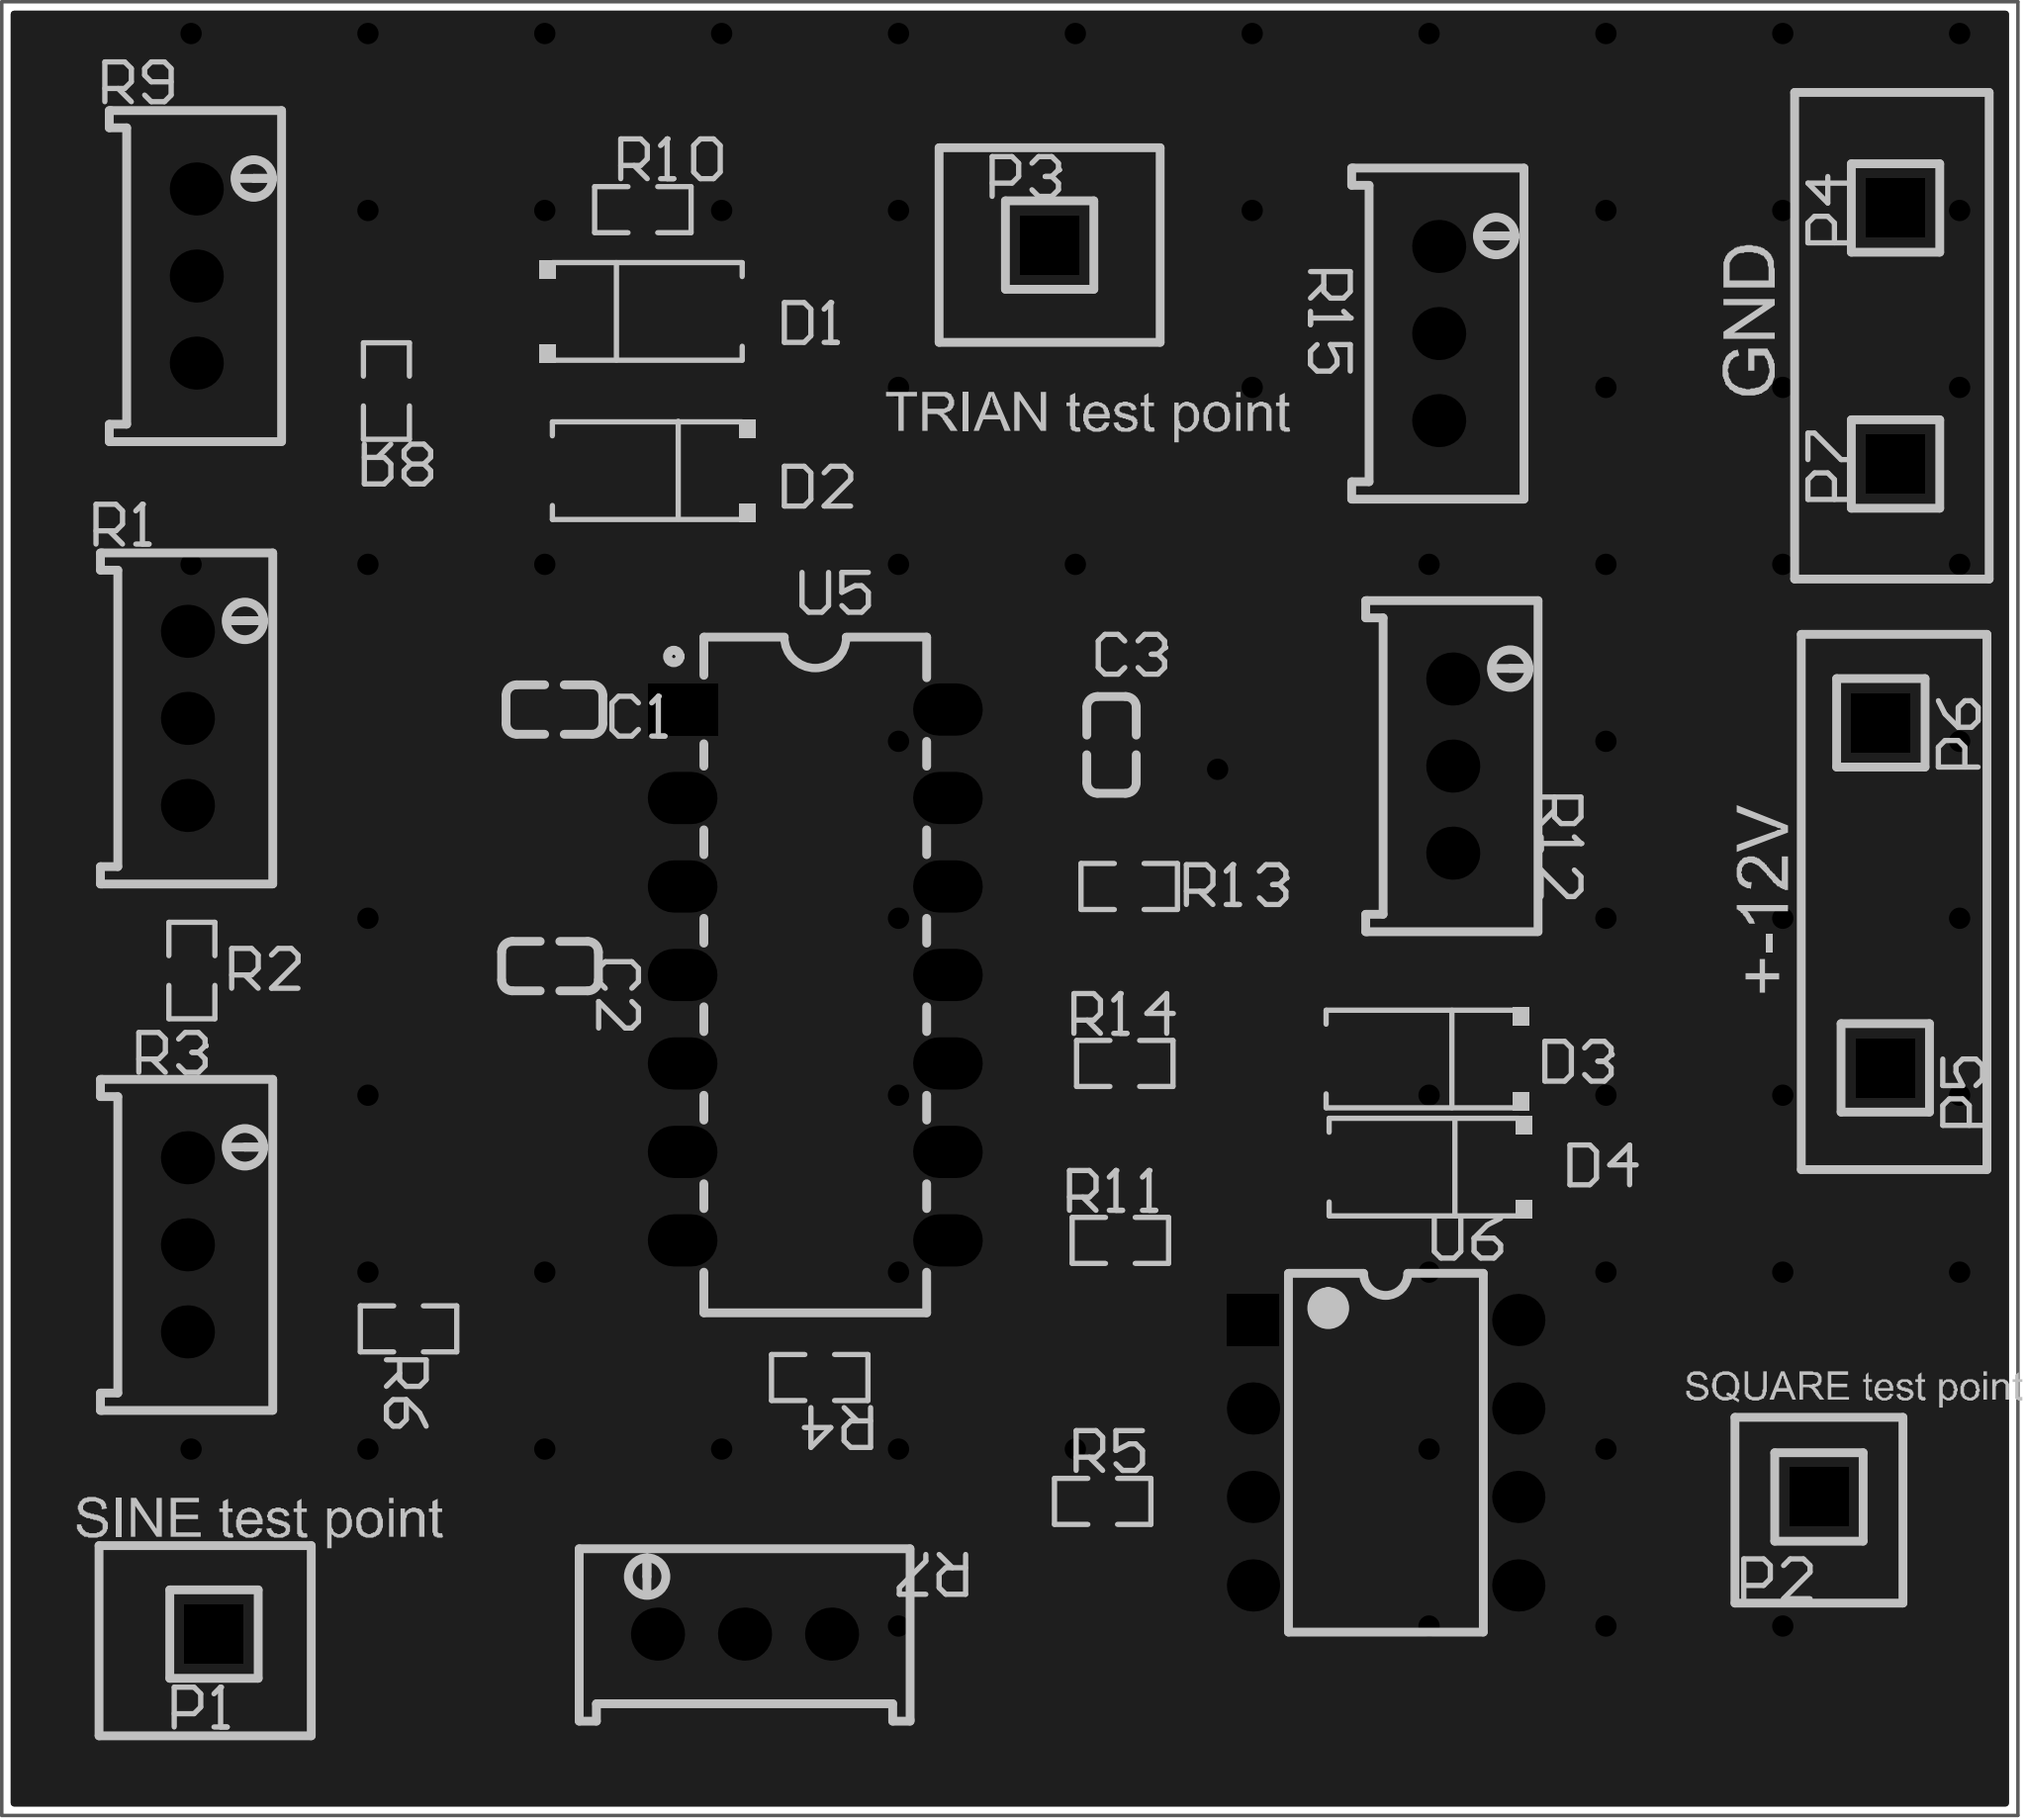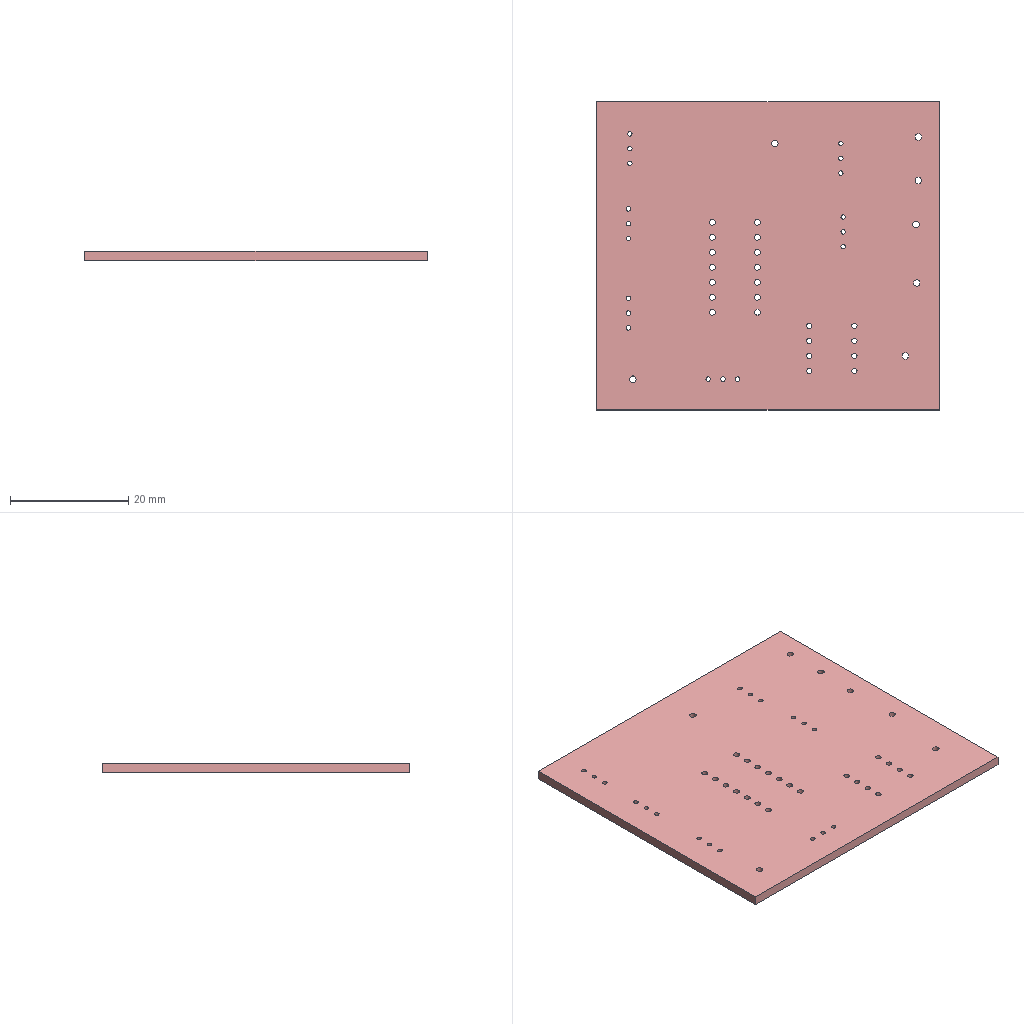Circuit board layout | Altium Designer | box 57.9 x 52.1 x 1.6 mm
Layer stack:
# Altium Designer layer stack of  (unit mm; dielectric type: 0 none, 1 core, 2 prepreg, 3 surface material)
index,name,kind,layer,copper_thickness_mm,dielectric_type,dielectric_thickness_mm,dielectric_material,dielectric_constant
0,Top Paste Mask Layer,other,,,,,,
1,Top Silkscreen Layer,other,,,,,,
2,Top Solder Mask Layer,dielectric,,,3,0.01,,3.3
3,Top Layer,copper,Top Layer,0.035,,,,
4,Dielectric1,dielectric,,,3,1.51,FR4,4.5
5,Bottom Layer,copper,Bottom Layer,0.035,,,,
6,Bottom Solder Mask Layer,dielectric,,,3,0.01,,3.3
7,Bottom Silkscreen Layer,other,,,,,,
8,Bottom Paste Mask Layer,other,,,,,,
# drill layer pairs: low layer,high layer
drill_pair,Top Layer,Bottom Layer
Part placement:
Designator,Comment,Layer,Footprint,Center-X(mm),Center-Y(mm),Rotation
C1,100nF,TopLayer,C0603,101.092,115.57,0
C2,100nF,TopLayer,C0603,100.965,108.204,0
C3,100nF,TopLayer,C0603,117.094,114.554,90
D3,1N4007,TopLayer,SMA_L4.3-W2.5-LS5.0-RD,125.984,105.537,180
D4,1N4007,TopLayer,SMA_L4.3-W2.5-LS5.0-RD,126.071,102.434,180
P1,2.54-1*1P pin,TopLayer,HDR-TH_1P-P2.54-V-M,91.313,89.027,0
P2,2.54-1*1P pin,TopLayer,HDR-TH_1P-P2.54-V-M,137.414,92.964,0
P3,2.54-1*1P pin,TopLayer,HDR-TH_1P-P2.54-V-M,115.316,128.905,0
P4,2.54-1*1P pin,TopLayer,HDR-TH_1P-P2.54-V-M,139.614,129.969,90
P5,2.54-1*1P pin,TopLayer,HDR-TH_1P-P2.54-V-M,139.319,105.283,90
P6,2.54-1*1P pin,TopLayer,HDR-TH_1P-P2.54-V-M,139.192,115.189,90
R1,50kΩ,TopLayer,RES-ADJ-TH_3P-L9.5-W4.85-P2.50-BL-BS,90.551,115.316,0
R2,5.1kΩ,TopLayer,R0603,90.678,108.077,90
R3,50kΩ,TopLayer,RES-ADJ-TH_3P-L9.5-W4.85-P2.50-BL-BS,90.551,100.203,0
R4,200Ω,TopLayer,R0603,108.712,96.393,180
R5,20kΩ,TopLayer,R0603,116.84,92.837,0
R6,5.1kΩ,TopLayer,R0603,96.901,97.79,180
R7,50kΩ,TopLayer,RES-ADJ-TH_3P-L9.5-W4.85-P2.50-BL-BS,106.553,89.027,90
R8,5.1kΩ,TopLayer,R0603,96.266,124.714,90
R9,50kΩ,TopLayer,RES-ADJ-TH_3P-L9.5-W4.85-P2.50-BL-BS,90.805,128.016,0
R10,5.1kΩ,TopLayer,R0603,103.632,129.921,0
R11,5.1kΩ,TopLayer,R0603,117.348,100.33,0
R12,50kΩ,TopLayer,RES-ADJ-TH_3P-L9.5-W4.85-P2.50-BL-BS,126.895,113.947,0
R13,5.1kΩ,TopLayer,R0603,117.602,110.49,180
R14,5.1kΩ,TopLayer,R0603,117.475,105.41,0
R15,50kΩ,TopLayer,RES-ADJ-TH_3P-L9.5-W4.85-P2.50-BL-BS,126.492,126.365,0
U5,LM324N,TopLayer,DIP-14_L19.4-W6.4-P2.54-LS7.6-BL,108.585,107.95,270
U6,LM741J,TopLayer,CDIP-8_L10.3-W6.7-P2.54-LS7.6-BL,124.968,94.234,270
D1,1N4007,TopLayer,SMA_L4.3-W2.5-LS5.0-RD,103.759,127,0
D2,1N4007,TopLayer,SMA_L4.3-W2.5-LS5.0-RD-1,103.759,122.428,180
P7,2.54-1*1P pin,TopLayer,HDR-TH_1P-P2.54-V-M,139.614,122.618,90
Pad and via stacks:
# Altium Designer via and pad stacks of  (unit mm). Each distinct definition once, with the count of objects using it.
# via: kind,start_layer,end_layer,hole_mm,diameter_mm,mode(0 simple;1 top-mid-bottom;2 full stack),diameter_per_layer,count,example_net
# pad: kind,layer,hole_mm,hole_type(0 round;1 square;2 slot),plating,top_size,top_shape(1 round;2 rect;3 octagon;9 rounded rect),mid_size,bottom_size,mode,footprint,size_per_layer,count,example
pad,Top Layer,0,0,plated,0.8x0.9,2,0.8x0.9,0.8x0.9,0,C0603,,6,C1.2
pad,Top Layer,0,0,plated,2x1.593,2,2x1.593,2x1.593,0,SMA_L4.3-W2.5-LS5.0-RD,,6,D3.2
pad,Top Layer,0,0,plated,0.8065x0.864,2,0.8065x0.864,0.8065x0.864,0,R0603,,18,R2.2
pad,Top Layer,0,0,plated,2.185x1.7,2,2.185x1.7,2.185x1.7,0,SMA_L4.3-W2.5-LS5.0-RD-1,,2,D2.1
pad,Multi-Layer,1.1,0,plated,1.7x1.7,2,1.7x1.7,1.7x1.7,0,HDR-TH_1P-P2.54-V-M,,7,P1.1
pad,Multi-Layer,0.762,0,plated,1.524x1.524,1,1.524x1.524,1.524x1.524,0,RES-ADJ-TH_3P-L9.5-W4.85-P2.50-BL-BS,,18,R1.2
pad,Multi-Layer,1,0,plated,2x1.5,1,2x1.5,2x1.5,0,DIP-14_L19.4-W6.4-P2.54-LS7.6-BL,,13,U5.8
pad,Multi-Layer,1,0,plated,2x1.5,2,2x1.5,2x1.5,0,DIP-14_L19.4-W6.4-P2.54-LS7.6-BL,,1,U5.1
pad,Multi-Layer,0.9,0,plated,1.5x1.5,2,1.5x1.5,1.5x1.5,0,CDIP-8_L10.3-W6.7-P2.54-LS7.6-BL,,1,U6.1
pad,Multi-Layer,0.9,0,plated,1.5x1.5,1,1.5x1.5,1.5x1.5,0,CDIP-8_L10.3-W6.7-P2.54-LS7.6-BL,,7,U6.2
via,Top Layer,Bottom Layer,0.3048,0.61,0,,67,$1N28
Copper pours:
name,layer,net,type(0 solid;1 hatched;2 none)
Top Layer-GND,Top Layer,GND,0
Bottom Layer-GND,Bottom Layer,GND,0
Design rules, without the lines most boards share:
# Altium Designer design rules of  (exported by Altium Designer, unit mm)
# columns: name | kind | enabled | priority | scope1 | scope2 | descriptor | typed fields (field=value)
solderMaskExpansion | 13 | enabled | 2 | All | All | Solder Mask Expansion (Expansion =2.008mil) (All) | expansion=0.051